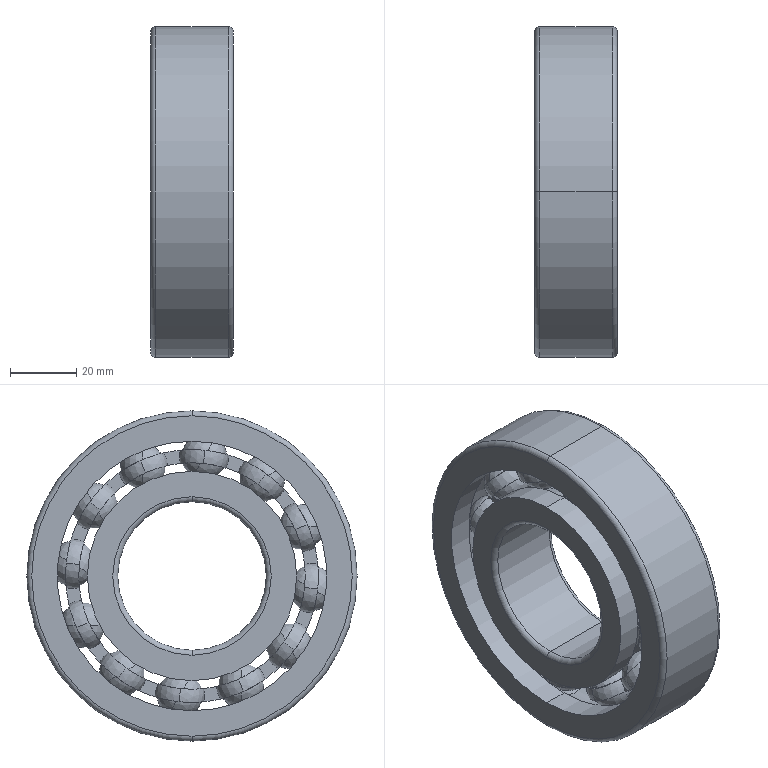Part | SolidWorks | features ReferencePattern 11, LocalCirPattern 1 | 15 solids | 154 faces | box 25 x 100 x 100 mm | volume 114868 mm3 | sphere 96 | plane 28 | cylinder 16 | torus 14 | commonest cylinder face diameters 63.4 x4 81.6 x4 45 x2 68.5 x2 76.5 x2 100 x2